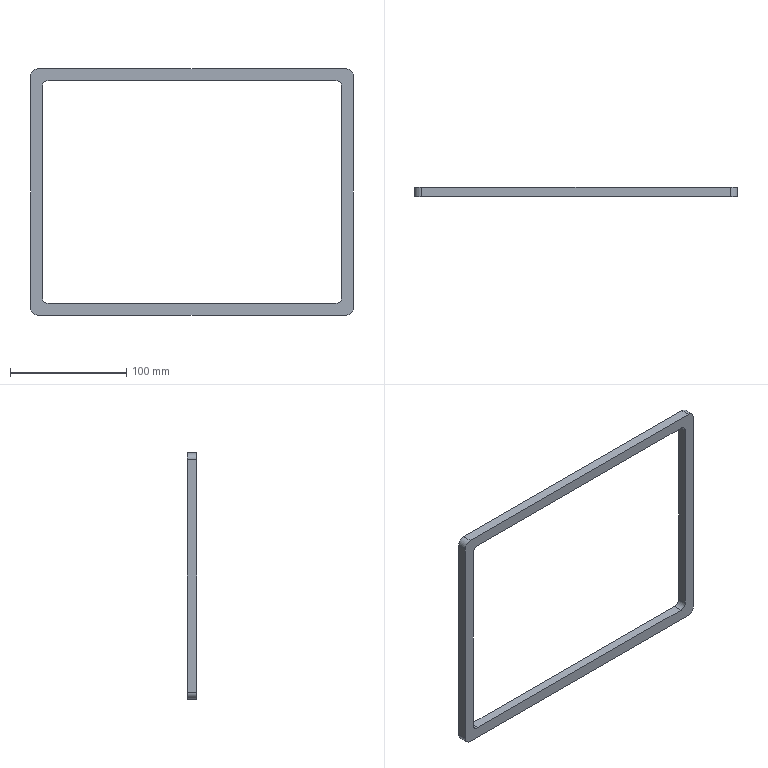Part | NX | 1 solid | 18 faces | box 278 x 8 x 212 mm | volume 75124 mm3 | plane 10 | cylinder 8 | commonest cylinder face diameters 10 x4 12 x4
STEP:
#1=CARTESIAN_POINT('',(-139.,4.,-100.));
#2=VERTEX_POINT('',#1);
#3=CARTESIAN_POINT('',(-133.,4.,-106.));
#4=VERTEX_POINT('',#3);
#5=CARTESIAN_POINT('',(-133.,4.,-100.));
#6=DIRECTION('',(0.,-1.,0.));
#7=DIRECTION('',(0.,0.,-1.));
#8=AXIS2_PLACEMENT_3D('',#5,#6,#7);
#9=CIRCLE('',#8,6.);
#10=EDGE_CURVE('',#2,#4,#9,.T.);
#11=ORIENTED_EDGE('',*,*,#10,.F.);
#12=CARTESIAN_POINT('',(-139.,4.,100.));
#13=VERTEX_POINT('',#12);
#14=CARTESIAN_POINT('',(-139.,4.,100.));
#15=DIRECTION('',(0.,0.,-1.));
#16=VECTOR('',#15,1000.);
#17=LINE('',#14,#16);
#18=EDGE_CURVE('',#13,#2,#17,.T.);
#19=ORIENTED_EDGE('',*,*,#18,.F.);
#20=CARTESIAN_POINT('',(-133.,4.,106.));
#21=VERTEX_POINT('',#20);
#22=CARTESIAN_POINT('',(-133.,4.,100.));
#23=DIRECTION('',(0.,-1.,0.));
#24=DIRECTION('',(0.,0.,-1.));
#25=AXIS2_PLACEMENT_3D('',#22,#23,#24);
#26=CIRCLE('',#25,6.);
#27=EDGE_CURVE('',#21,#13,#26,.T.);
#28=ORIENTED_EDGE('',*,*,#27,.F.);
#29=CARTESIAN_POINT('',(133.,4.,106.));
#30=VERTEX_POINT('',#29);
#31=CARTESIAN_POINT('',(133.,4.,106.));
#32=DIRECTION('',(-1.,0.,0.));
#33=VECTOR('',#32,1000.);
#34=LINE('',#31,#33);
#35=EDGE_CURVE('',#30,#21,#34,.T.);
#36=ORIENTED_EDGE('',*,*,#35,.F.);
#37=CARTESIAN_POINT('',(139.,4.,100.));
#38=VERTEX_POINT('',#37);
#39=CARTESIAN_POINT('',(133.,4.,100.));
#40=DIRECTION('',(0.,-1.,0.));
#41=DIRECTION('',(0.,0.,-1.));
#42=AXIS2_PLACEMENT_3D('',#39,#40,#41);
#43=CIRCLE('',#42,6.);
#44=EDGE_CURVE('',#38,#30,#43,.T.);
#45=ORIENTED_EDGE('',*,*,#44,.F.);
#46=CARTESIAN_POINT('',(139.,4.,-100.));
#47=VERTEX_POINT('',#46);
#48=CARTESIAN_POINT('',(139.,4.,-100.));
#49=DIRECTION('',(0.,0.,1.));
#50=VECTOR('',#49,1000.);
#51=LINE('',#48,#50);
#52=EDGE_CURVE('',#47,#38,#51,.T.);
#53=ORIENTED_EDGE('',*,*,#52,.F.);
#54=CARTESIAN_POINT('',(133.,4.,-106.));
#55=VERTEX_POINT('',#54);
#56=CARTESIAN_POINT('',(133.,4.,-100.));
#57=DIRECTION('',(0.,-1.,0.));
#58=DIRECTION('',(0.,0.,-1.));
#59=AXIS2_PLACEMENT_3D('',#56,#57,#58);
#60=CIRCLE('',#59,6.);
#61=EDGE_CURVE('',#55,#47,#60,.T.);
#62=ORIENTED_EDGE('',*,*,#61,.F.);
#63=CARTESIAN_POINT('',(-133.,4.,-106.));
#64=DIRECTION('',(1.,0.,0.));
#65=VECTOR('',#64,1000.);
#66=LINE('',#63,#65);
#67=EDGE_CURVE('',#4,#55,#66,.T.);
#68=ORIENTED_EDGE('',*,*,#67,.F.);
#69=EDGE_LOOP('',(#11,#19,#28,#36,#45,#53,#62,#68));
#70=FACE_BOUND('',#69,.T.);
#71=CARTESIAN_POINT('',(-129.,4.,-91.));
#72=VERTEX_POINT('',#71);
#73=CARTESIAN_POINT('',(-124.,4.,-96.));
#74=VERTEX_POINT('',#73);
#75=CARTESIAN_POINT('',(-124.,4.,-91.));
#76=DIRECTION('',(0.,-1.,0.));
#77=DIRECTION('',(0.,0.,-1.));
#78=AXIS2_PLACEMENT_3D('',#75,#76,#77);
#79=CIRCLE('',#78,5.);
#80=EDGE_CURVE('',#72,#74,#79,.T.);
#81=ORIENTED_EDGE('',*,*,#80,.T.);
#82=CARTESIAN_POINT('',(124.,4.,-96.));
#83=VERTEX_POINT('',#82);
#84=CARTESIAN_POINT('',(-124.,4.,-96.));
#85=DIRECTION('',(1.,0.,0.));
#86=VECTOR('',#85,1000.);
#87=LINE('',#84,#86);
#88=EDGE_CURVE('',#74,#83,#87,.T.);
#89=ORIENTED_EDGE('',*,*,#88,.T.);
#90=CARTESIAN_POINT('',(129.,4.,-91.));
#91=VERTEX_POINT('',#90);
#92=CARTESIAN_POINT('',(124.,4.,-91.));
#93=DIRECTION('',(0.,-1.,0.));
#94=DIRECTION('',(0.,0.,-1.));
#95=AXIS2_PLACEMENT_3D('',#92,#93,#94);
#96=CIRCLE('',#95,5.);
#97=EDGE_CURVE('',#83,#91,#96,.T.);
#98=ORIENTED_EDGE('',*,*,#97,.T.);
#99=CARTESIAN_POINT('',(129.,4.,91.));
#100=VERTEX_POINT('',#99);
#101=CARTESIAN_POINT('',(129.,4.,-91.));
#102=DIRECTION('',(0.,0.,1.));
#103=VECTOR('',#102,1000.);
#104=LINE('',#101,#103);
#105=EDGE_CURVE('',#91,#100,#104,.T.);
#106=ORIENTED_EDGE('',*,*,#105,.T.);
#107=CARTESIAN_POINT('',(124.,4.,96.));
#108=VERTEX_POINT('',#107);
#109=CARTESIAN_POINT('',(124.,4.,91.));
#110=DIRECTION('',(0.,-1.,0.));
#111=DIRECTION('',(0.,0.,-1.));
#112=AXIS2_PLACEMENT_3D('',#109,#110,#111);
#113=CIRCLE('',#112,5.);
#114=EDGE_CURVE('',#100,#108,#113,.T.);
#115=ORIENTED_EDGE('',*,*,#114,.T.);
#116=CARTESIAN_POINT('',(-124.,4.,96.));
#117=VERTEX_POINT('',#116);
#118=CARTESIAN_POINT('',(124.,4.,96.));
#119=DIRECTION('',(-1.,0.,0.));
#120=VECTOR('',#119,1000.);
#121=LINE('',#118,#120);
#122=EDGE_CURVE('',#108,#117,#121,.T.);
#123=ORIENTED_EDGE('',*,*,#122,.T.);
#124=CARTESIAN_POINT('',(-129.,4.,91.));
#125=VERTEX_POINT('',#124);
#126=CARTESIAN_POINT('',(-124.,4.,91.));
#127=DIRECTION('',(0.,-1.,0.));
#128=DIRECTION('',(0.,0.,-1.));
#129=AXIS2_PLACEMENT_3D('',#126,#127,#128);
#130=CIRCLE('',#129,5.);
#131=EDGE_CURVE('',#117,#125,#130,.T.);
#132=ORIENTED_EDGE('',*,*,#131,.T.);
#133=CARTESIAN_POINT('',(-129.,4.,91.));
#134=DIRECTION('',(0.,0.,-1.));
#135=VECTOR('',#134,1000.);
#136=LINE('',#133,#135);
#137=EDGE_CURVE('',#125,#72,#136,.T.);
#138=ORIENTED_EDGE('',*,*,#137,.T.);
#139=EDGE_LOOP('',(#81,#89,#98,#106,#115,#123,#132,#138));
#140=FACE_BOUND('',#139,.T.);
#141=CARTESIAN_POINT('',(-133.,4.,-100.));
#142=DIRECTION('',(0.,-1.,0.));
#143=DIRECTION('',(0.,0.,-1.));
#144=AXIS2_PLACEMENT_3D('',#141,#142,#143);
#145=PLANE('',#144);
#146=ADVANCED_FACE('',(#70,#140),#145,.F.);
#147=CARTESIAN_POINT('',(-133.,-4.,-106.));
#148=VERTEX_POINT('',#147);
#149=CARTESIAN_POINT('',(-133.,-353.611,-106.));
#150=DIRECTION('',(0.,1.,0.));
#151=VECTOR('',#150,1000.);
#152=LINE('',#149,#151);
#153=EDGE_CURVE('',#148,#4,#152,.T.);
#154=ORIENTED_EDGE('',*,*,#153,.F.);
#155=CARTESIAN_POINT('',(-139.,-4.,-100.));
#156=VERTEX_POINT('',#155);
#157=CARTESIAN_POINT('',(-133.,-4.,-100.));
#158=DIRECTION('',(0.,1.,0.));
#159=DIRECTION('',(0.,0.,1.));
#160=AXIS2_PLACEMENT_3D('',#157,#158,#159);
#161=CIRCLE('',#160,6.);
#162=EDGE_CURVE('',#148,#156,#161,.T.);
#163=ORIENTED_EDGE('',*,*,#162,.T.);
#164=CARTESIAN_POINT('',(-139.,-353.611,-100.));
#165=DIRECTION('',(0.,1.,0.));
#166=VECTOR('',#165,1000.);
#167=LINE('',#164,#166);
#168=EDGE_CURVE('',#156,#2,#167,.T.);
#169=ORIENTED_EDGE('',*,*,#168,.T.);
#170=ORIENTED_EDGE('',*,*,#10,.T.);
#171=EDGE_LOOP('',(#154,#163,#169,#170));
#172=FACE_BOUND('',#171,.T.);
#173=CARTESIAN_POINT('',(-133.,-353.611,-100.));
#174=DIRECTION('',(0.,1.,0.));
#175=DIRECTION('',(0.,0.,1.));
#176=AXIS2_PLACEMENT_3D('',#173,#174,#175);
#177=CYLINDRICAL_SURFACE('',#176,6.);
#178=ADVANCED_FACE('',(#172),#177,.T.);
#179=CARTESIAN_POINT('',(133.,-4.,-106.));
#180=VERTEX_POINT('',#179);
#181=CARTESIAN_POINT('',(133.,-353.611,-106.));
#182=DIRECTION('',(0.,1.,0.));
#183=VECTOR('',#182,1000.);
#184=LINE('',#181,#183);
#185=EDGE_CURVE('',#180,#55,#184,.T.);
#186=ORIENTED_EDGE('',*,*,#185,.F.);
#187=CARTESIAN_POINT('',(-133.,-4.,-106.));
#188=DIRECTION('',(-1.,0.,0.));
#189=VECTOR('',#188,1000.);
#190=LINE('',#187,#189);
#191=EDGE_CURVE('',#180,#148,#190,.T.);
#192=ORIENTED_EDGE('',*,*,#191,.T.);
#193=ORIENTED_EDGE('',*,*,#153,.T.);
#194=ORIENTED_EDGE('',*,*,#67,.T.);
#195=EDGE_LOOP('',(#186,#192,#193,#194));
#196=FACE_BOUND('',#195,.T.);
#197=CARTESIAN_POINT('',(-133.,-353.611,-106.));
#198=DIRECTION('',(0.,0.,1.));
#199=DIRECTION('',(1.,0.,0.));
#200=AXIS2_PLACEMENT_3D('',#197,#198,#199);
#201=PLANE('',#200);
#202=ADVANCED_FACE('',(#196),#201,.F.);
#203=CARTESIAN_POINT('',(139.,-4.,-100.));
#204=VERTEX_POINT('',#203);
#205=CARTESIAN_POINT('',(139.,-353.611,-100.));
#206=DIRECTION('',(0.,1.,0.));
#207=VECTOR('',#206,1000.);
#208=LINE('',#205,#207);
#209=EDGE_CURVE('',#204,#47,#208,.T.);
#210=ORIENTED_EDGE('',*,*,#209,.F.);
#211=CARTESIAN_POINT('',(133.,-4.,-100.));
#212=DIRECTION('',(0.,1.,0.));
#213=DIRECTION('',(0.,0.,1.));
#214=AXIS2_PLACEMENT_3D('',#211,#212,#213);
#215=CIRCLE('',#214,6.);
#216=EDGE_CURVE('',#204,#180,#215,.T.);
#217=ORIENTED_EDGE('',*,*,#216,.T.);
#218=ORIENTED_EDGE('',*,*,#185,.T.);
#219=ORIENTED_EDGE('',*,*,#61,.T.);
#220=EDGE_LOOP('',(#210,#217,#218,#219));
#221=FACE_BOUND('',#220,.T.);
#222=CARTESIAN_POINT('',(133.,-353.611,-100.));
#223=DIRECTION('',(0.,1.,0.));
#224=DIRECTION('',(0.,0.,1.));
#225=AXIS2_PLACEMENT_3D('',#222,#223,#224);
#226=CYLINDRICAL_SURFACE('',#225,6.);
#227=ADVANCED_FACE('',(#221),#226,.T.);
#228=CARTESIAN_POINT('',(139.,-4.,100.));
#229=VERTEX_POINT('',#228);
#230=CARTESIAN_POINT('',(139.,-353.611,100.));
#231=DIRECTION('',(0.,1.,0.));
#232=VECTOR('',#231,1000.);
#233=LINE('',#230,#232);
#234=EDGE_CURVE('',#229,#38,#233,.T.);
#235=ORIENTED_EDGE('',*,*,#234,.F.);
#236=CARTESIAN_POINT('',(139.,-4.,-100.));
#237=DIRECTION('',(0.,0.,-1.));
#238=VECTOR('',#237,1000.);
#239=LINE('',#236,#238);
#240=EDGE_CURVE('',#229,#204,#239,.T.);
#241=ORIENTED_EDGE('',*,*,#240,.T.);
#242=ORIENTED_EDGE('',*,*,#209,.T.);
#243=ORIENTED_EDGE('',*,*,#52,.T.);
#244=EDGE_LOOP('',(#235,#241,#242,#243));
#245=FACE_BOUND('',#244,.T.);
#246=CARTESIAN_POINT('',(139.,-353.611,-100.));
#247=DIRECTION('',(-1.,0.,0.));
#248=DIRECTION('',(0.,0.,1.));
#249=AXIS2_PLACEMENT_3D('',#246,#247,#248);
#250=PLANE('',#249);
#251=ADVANCED_FACE('',(#245),#250,.F.);
#252=CARTESIAN_POINT('',(133.,-4.,106.));
#253=VERTEX_POINT('',#252);
#254=CARTESIAN_POINT('',(133.,-353.611,106.));
#255=DIRECTION('',(0.,1.,0.));
#256=VECTOR('',#255,1000.);
#257=LINE('',#254,#256);
#258=EDGE_CURVE('',#253,#30,#257,.T.);
#259=ORIENTED_EDGE('',*,*,#258,.F.);
#260=CARTESIAN_POINT('',(133.,-4.,100.));
#261=DIRECTION('',(0.,1.,0.));
#262=DIRECTION('',(0.,0.,1.));
#263=AXIS2_PLACEMENT_3D('',#260,#261,#262);
#264=CIRCLE('',#263,6.);
#265=EDGE_CURVE('',#253,#229,#264,.T.);
#266=ORIENTED_EDGE('',*,*,#265,.T.);
#267=ORIENTED_EDGE('',*,*,#234,.T.);
#268=ORIENTED_EDGE('',*,*,#44,.T.);
#269=EDGE_LOOP('',(#259,#266,#267,#268));
#270=FACE_BOUND('',#269,.T.);
#271=CARTESIAN_POINT('',(133.,-353.611,100.));
#272=DIRECTION('',(0.,1.,0.));
#273=DIRECTION('',(0.,0.,1.));
#274=AXIS2_PLACEMENT_3D('',#271,#272,#273);
#275=CYLINDRICAL_SURFACE('',#274,6.);
#276=ADVANCED_FACE('',(#270),#275,.T.);
#277=CARTESIAN_POINT('',(-133.,-4.,106.));
#278=VERTEX_POINT('',#277);
#279=CARTESIAN_POINT('',(-133.,-353.611,106.));
#280=DIRECTION('',(0.,1.,0.));
#281=VECTOR('',#280,1000.);
#282=LINE('',#279,#281);
#283=EDGE_CURVE('',#278,#21,#282,.T.);
#284=ORIENTED_EDGE('',*,*,#283,.F.);
#285=CARTESIAN_POINT('',(133.,-4.,106.));
#286=DIRECTION('',(1.,0.,0.));
#287=VECTOR('',#286,1000.);
#288=LINE('',#285,#287);
#289=EDGE_CURVE('',#278,#253,#288,.T.);
#290=ORIENTED_EDGE('',*,*,#289,.T.);
#291=ORIENTED_EDGE('',*,*,#258,.T.);
#292=ORIENTED_EDGE('',*,*,#35,.T.);
#293=EDGE_LOOP('',(#284,#290,#291,#292));
#294=FACE_BOUND('',#293,.T.);
#295=CARTESIAN_POINT('',(133.,-353.611,106.));
#296=DIRECTION('',(0.,0.,-1.));
#297=DIRECTION('',(-1.,0.,0.));
#298=AXIS2_PLACEMENT_3D('',#295,#296,#297);
#299=PLANE('',#298);
#300=ADVANCED_FACE('',(#294),#299,.F.);
#301=CARTESIAN_POINT('',(-139.,-4.,100.));
#302=VERTEX_POINT('',#301);
#303=CARTESIAN_POINT('',(-139.,-353.611,100.));
#304=DIRECTION('',(0.,1.,0.));
#305=VECTOR('',#304,1000.);
#306=LINE('',#303,#305);
#307=EDGE_CURVE('',#302,#13,#306,.T.);
#308=ORIENTED_EDGE('',*,*,#307,.F.);
#309=CARTESIAN_POINT('',(-133.,-4.,100.));
#310=DIRECTION('',(0.,1.,0.));
#311=DIRECTION('',(0.,0.,1.));
#312=AXIS2_PLACEMENT_3D('',#309,#310,#311);
#313=CIRCLE('',#312,6.);
#314=EDGE_CURVE('',#302,#278,#313,.T.);
#315=ORIENTED_EDGE('',*,*,#314,.T.);
#316=ORIENTED_EDGE('',*,*,#283,.T.);
#317=ORIENTED_EDGE('',*,*,#27,.T.);
#318=EDGE_LOOP('',(#308,#315,#316,#317));
#319=FACE_BOUND('',#318,.T.);
#320=CARTESIAN_POINT('',(-133.,-353.611,100.));
#321=DIRECTION('',(0.,1.,0.));
#322=DIRECTION('',(0.,0.,1.));
#323=AXIS2_PLACEMENT_3D('',#320,#321,#322);
#324=CYLINDRICAL_SURFACE('',#323,6.);
#325=ADVANCED_FACE('',(#319),#324,.T.);
#326=ORIENTED_EDGE('',*,*,#168,.F.);
#327=CARTESIAN_POINT('',(-139.,-4.,100.));
#328=DIRECTION('',(0.,0.,1.));
#329=VECTOR('',#328,1000.);
#330=LINE('',#327,#329);
#331=EDGE_CURVE('',#156,#302,#330,.T.);
#332=ORIENTED_EDGE('',*,*,#331,.T.);
#333=ORIENTED_EDGE('',*,*,#307,.T.);
#334=ORIENTED_EDGE('',*,*,#18,.T.);
#335=EDGE_LOOP('',(#326,#332,#333,#334));
#336=FACE_BOUND('',#335,.T.);
#337=CARTESIAN_POINT('',(-139.,-353.611,100.));
#338=DIRECTION('',(1.,0.,0.));
#339=DIRECTION('',(0.,0.,-1.));
#340=AXIS2_PLACEMENT_3D('',#337,#338,#339);
#341=PLANE('',#340);
#342=ADVANCED_FACE('',(#336),#341,.F.);
#343=CARTESIAN_POINT('',(-124.,-4.,-96.));
#344=VERTEX_POINT('',#343);
#345=CARTESIAN_POINT('',(-129.,-4.,-91.));
#346=VERTEX_POINT('',#345);
#347=CARTESIAN_POINT('',(-124.,-4.,-91.));
#348=DIRECTION('',(0.,1.,0.));
#349=DIRECTION('',(0.,0.,1.));
#350=AXIS2_PLACEMENT_3D('',#347,#348,#349);
#351=CIRCLE('',#350,5.);
#352=EDGE_CURVE('',#344,#346,#351,.T.);
#353=ORIENTED_EDGE('',*,*,#352,.F.);
#354=CARTESIAN_POINT('',(-124.,-353.611,-96.));
#355=DIRECTION('',(0.,1.,0.));
#356=VECTOR('',#355,1000.);
#357=LINE('',#354,#356);
#358=EDGE_CURVE('',#344,#74,#357,.T.);
#359=ORIENTED_EDGE('',*,*,#358,.T.);
#360=ORIENTED_EDGE('',*,*,#80,.F.);
#361=CARTESIAN_POINT('',(-129.,-353.611,-91.));
#362=DIRECTION('',(0.,1.,0.));
#363=VECTOR('',#362,1000.);
#364=LINE('',#361,#363);
#365=EDGE_CURVE('',#346,#72,#364,.T.);
#366=ORIENTED_EDGE('',*,*,#365,.F.);
#367=EDGE_LOOP('',(#353,#359,#360,#366));
#368=FACE_BOUND('',#367,.T.);
#369=CARTESIAN_POINT('',(-124.,-353.611,-91.));
#370=DIRECTION('',(0.,1.,0.));
#371=DIRECTION('',(0.,0.,1.));
#372=AXIS2_PLACEMENT_3D('',#369,#370,#371);
#373=CYLINDRICAL_SURFACE('',#372,5.);
#374=ADVANCED_FACE('',(#368),#373,.F.);
#375=CARTESIAN_POINT('',(124.,-4.,-96.));
#376=VERTEX_POINT('',#375);
#377=CARTESIAN_POINT('',(-124.,-4.,-96.));
#378=DIRECTION('',(-1.,0.,0.));
#379=VECTOR('',#378,1000.);
#380=LINE('',#377,#379);
#381=EDGE_CURVE('',#376,#344,#380,.T.);
#382=ORIENTED_EDGE('',*,*,#381,.F.);
#383=CARTESIAN_POINT('',(124.,-353.611,-96.));
#384=DIRECTION('',(0.,1.,0.));
#385=VECTOR('',#384,1000.);
#386=LINE('',#383,#385);
#387=EDGE_CURVE('',#376,#83,#386,.T.);
#388=ORIENTED_EDGE('',*,*,#387,.T.);
#389=ORIENTED_EDGE('',*,*,#88,.F.);
#390=ORIENTED_EDGE('',*,*,#358,.F.);
#391=EDGE_LOOP('',(#382,#388,#389,#390));
#392=FACE_BOUND('',#391,.T.);
#393=CARTESIAN_POINT('',(-124.,-353.611,-96.));
#394=DIRECTION('',(0.,0.,1.));
#395=DIRECTION('',(1.,0.,0.));
#396=AXIS2_PLACEMENT_3D('',#393,#394,#395);
#397=PLANE('',#396);
#398=ADVANCED_FACE('',(#392),#397,.T.);
#399=CARTESIAN_POINT('',(129.,-4.,-91.));
#400=VERTEX_POINT('',#399);
#401=CARTESIAN_POINT('',(124.,-4.,-91.));
#402=DIRECTION('',(0.,1.,0.));
#403=DIRECTION('',(0.,0.,1.));
#404=AXIS2_PLACEMENT_3D('',#401,#402,#403);
#405=CIRCLE('',#404,5.);
#406=EDGE_CURVE('',#400,#376,#405,.T.);
#407=ORIENTED_EDGE('',*,*,#406,.F.);
#408=CARTESIAN_POINT('',(129.,-353.611,-91.));
#409=DIRECTION('',(0.,1.,0.));
#410=VECTOR('',#409,1000.);
#411=LINE('',#408,#410);
#412=EDGE_CURVE('',#400,#91,#411,.T.);
#413=ORIENTED_EDGE('',*,*,#412,.T.);
#414=ORIENTED_EDGE('',*,*,#97,.F.);
#415=ORIENTED_EDGE('',*,*,#387,.F.);
#416=EDGE_LOOP('',(#407,#413,#414,#415));
#417=FACE_BOUND('',#416,.T.);
#418=CARTESIAN_POINT('',(124.,-353.611,-91.));
#419=DIRECTION('',(0.,1.,0.));
#420=DIRECTION('',(0.,0.,1.));
#421=AXIS2_PLACEMENT_3D('',#418,#419,#420);
#422=CYLINDRICAL_SURFACE('',#421,5.);
#423=ADVANCED_FACE('',(#417),#422,.F.);
#424=CARTESIAN_POINT('',(129.,-4.,91.));
#425=VERTEX_POINT('',#424);
#426=CARTESIAN_POINT('',(129.,-4.,-91.));
#427=DIRECTION('',(0.,0.,-1.));
#428=VECTOR('',#427,1000.);
#429=LINE('',#426,#428);
#430=EDGE_CURVE('',#425,#400,#429,.T.);
#431=ORIENTED_EDGE('',*,*,#430,.F.);
#432=CARTESIAN_POINT('',(129.,-353.611,91.));
#433=DIRECTION('',(0.,1.,0.));
#434=VECTOR('',#433,1000.);
#435=LINE('',#432,#434);
#436=EDGE_CURVE('',#425,#100,#435,.T.);
#437=ORIENTED_EDGE('',*,*,#436,.T.);
#438=ORIENTED_EDGE('',*,*,#105,.F.);
#439=ORIENTED_EDGE('',*,*,#412,.F.);
#440=EDGE_LOOP('',(#431,#437,#438,#439));
#441=FACE_BOUND('',#440,.T.);
#442=CARTESIAN_POINT('',(129.,-353.611,-91.));
#443=DIRECTION('',(-1.,0.,0.));
#444=DIRECTION('',(0.,0.,1.));
#445=AXIS2_PLACEMENT_3D('',#442,#443,#444);
#446=PLANE('',#445);
#447=ADVANCED_FACE('',(#441),#446,.T.);
#448=CARTESIAN_POINT('',(124.,-4.,96.));
#449=VERTEX_POINT('',#448);
#450=CARTESIAN_POINT('',(124.,-4.,91.));
#451=DIRECTION('',(0.,1.,0.));
#452=DIRECTION('',(0.,0.,1.));
#453=AXIS2_PLACEMENT_3D('',#450,#451,#452);
#454=CIRCLE('',#453,5.);
#455=EDGE_CURVE('',#449,#425,#454,.T.);
#456=ORIENTED_EDGE('',*,*,#455,.F.);
#457=CARTESIAN_POINT('',(124.,-353.611,96.));
#458=DIRECTION('',(0.,1.,0.));
#459=VECTOR('',#458,1000.);
#460=LINE('',#457,#459);
#461=EDGE_CURVE('',#449,#108,#460,.T.);
#462=ORIENTED_EDGE('',*,*,#461,.T.);
#463=ORIENTED_EDGE('',*,*,#114,.F.);
#464=ORIENTED_EDGE('',*,*,#436,.F.);
#465=EDGE_LOOP('',(#456,#462,#463,#464));
#466=FACE_BOUND('',#465,.T.);
#467=CARTESIAN_POINT('',(124.,-353.611,91.));
#468=DIRECTION('',(0.,1.,0.));
#469=DIRECTION('',(0.,0.,1.));
#470=AXIS2_PLACEMENT_3D('',#467,#468,#469);
#471=CYLINDRICAL_SURFACE('',#470,5.);
#472=ADVANCED_FACE('',(#466),#471,.F.);
#473=CARTESIAN_POINT('',(-124.,-4.,96.));
#474=VERTEX_POINT('',#473);
#475=CARTESIAN_POINT('',(124.,-4.,96.));
#476=DIRECTION('',(1.,0.,0.));
#477=VECTOR('',#476,1000.);
#478=LINE('',#475,#477);
#479=EDGE_CURVE('',#474,#449,#478,.T.);
#480=ORIENTED_EDGE('',*,*,#479,.F.);
#481=CARTESIAN_POINT('',(-124.,-353.611,96.));
#482=DIRECTION('',(0.,1.,0.));
#483=VECTOR('',#482,1000.);
#484=LINE('',#481,#483);
#485=EDGE_CURVE('',#474,#117,#484,.T.);
#486=ORIENTED_EDGE('',*,*,#485,.T.);
#487=ORIENTED_EDGE('',*,*,#122,.F.);
#488=ORIENTED_EDGE('',*,*,#461,.F.);
#489=EDGE_LOOP('',(#480,#486,#487,#488));
#490=FACE_BOUND('',#489,.T.);
#491=CARTESIAN_POINT('',(124.,-353.611,96.));
#492=DIRECTION('',(0.,0.,-1.));
#493=DIRECTION('',(-1.,0.,0.));
#494=AXIS2_PLACEMENT_3D('',#491,#492,#493);
#495=PLANE('',#494);
#496=ADVANCED_FACE('',(#490),#495,.T.);
#497=CARTESIAN_POINT('',(-129.,-4.,91.));
#498=VERTEX_POINT('',#497);
#499=CARTESIAN_POINT('',(-124.,-4.,91.));
#500=DIRECTION('',(0.,1.,0.));
#501=DIRECTION('',(0.,0.,1.));
#502=AXIS2_PLACEMENT_3D('',#499,#500,#501);
#503=CIRCLE('',#502,5.);
#504=EDGE_CURVE('',#498,#474,#503,.T.);
#505=ORIENTED_EDGE('',*,*,#504,.F.);
#506=CARTESIAN_POINT('',(-129.,-353.611,91.));
#507=DIRECTION('',(0.,1.,0.));
#508=VECTOR('',#507,1000.);
#509=LINE('',#506,#508);
#510=EDGE_CURVE('',#498,#125,#509,.T.);
#511=ORIENTED_EDGE('',*,*,#510,.T.);
#512=ORIENTED_EDGE('',*,*,#131,.F.);
#513=ORIENTED_EDGE('',*,*,#485,.F.);
#514=EDGE_LOOP('',(#505,#511,#512,#513));
#515=FACE_BOUND('',#514,.T.);
#516=CARTESIAN_POINT('',(-124.,-353.611,91.));
#517=DIRECTION('',(0.,1.,0.));
#518=DIRECTION('',(0.,0.,1.));
#519=AXIS2_PLACEMENT_3D('',#516,#517,#518);
#520=CYLINDRICAL_SURFACE('',#519,5.);
#521=ADVANCED_FACE('',(#515),#520,.F.);
#522=CARTESIAN_POINT('',(-129.,-4.,91.));
#523=DIRECTION('',(0.,0.,1.));
#524=VECTOR('',#523,1000.);
#525=LINE('',#522,#524);
#526=EDGE_CURVE('',#346,#498,#525,.T.);
#527=ORIENTED_EDGE('',*,*,#526,.F.);
#528=ORIENTED_EDGE('',*,*,#365,.T.);
#529=ORIENTED_EDGE('',*,*,#137,.F.);
#530=ORIENTED_EDGE('',*,*,#510,.F.);
#531=EDGE_LOOP('',(#527,#528,#529,#530));
#532=FACE_BOUND('',#531,.T.);
#533=CARTESIAN_POINT('',(-129.,-353.611,91.));
#534=DIRECTION('',(1.,0.,0.));
#535=DIRECTION('',(0.,0.,-1.));
#536=AXIS2_PLACEMENT_3D('',#533,#534,#535);
#537=PLANE('',#536);
#538=ADVANCED_FACE('',(#532),#537,.T.);
#539=ORIENTED_EDGE('',*,*,#352,.T.);
#540=ORIENTED_EDGE('',*,*,#526,.T.);
#541=ORIENTED_EDGE('',*,*,#504,.T.);
#542=ORIENTED_EDGE('',*,*,#479,.T.);
#543=ORIENTED_EDGE('',*,*,#455,.T.);
#544=ORIENTED_EDGE('',*,*,#430,.T.);
#545=ORIENTED_EDGE('',*,*,#406,.T.);
#546=ORIENTED_EDGE('',*,*,#381,.T.);
#547=EDGE_LOOP('',(#539,#540,#541,#542,#543,#544,#545,#546));
#548=FACE_BOUND('',#547,.T.);
#549=ORIENTED_EDGE('',*,*,#191,.F.);
#550=ORIENTED_EDGE('',*,*,#216,.F.);
#551=ORIENTED_EDGE('',*,*,#240,.F.);
#552=ORIENTED_EDGE('',*,*,#265,.F.);
#553=ORIENTED_EDGE('',*,*,#289,.F.);
#554=ORIENTED_EDGE('',*,*,#314,.F.);
#555=ORIENTED_EDGE('',*,*,#331,.F.);
#556=ORIENTED_EDGE('',*,*,#162,.F.);
#557=EDGE_LOOP('',(#549,#550,#551,#552,#553,#554,#555,#556));
#558=FACE_BOUND('',#557,.T.);
#559=CARTESIAN_POINT('',(0.,-4.,0.));
#560=DIRECTION('',(0.,1.,0.));
#561=DIRECTION('',(0.,0.,1.));
#562=AXIS2_PLACEMENT_3D('',#559,#560,#561);
#563=PLANE('',#562);
#564=ADVANCED_FACE('',(#548,#558),#563,.F.);
#565=CLOSED_SHELL('',(#146,#178,#202,#227,#251,#276,#300,#325,#342,#374,#398,#423,#447,#472,#496,#521,#538,#564));
#566=MANIFOLD_SOLID_BREP('',#565);
#567=(LENGTH_UNIT()NAMED_UNIT(*)SI_UNIT(.MILLI.,.METRE.));
#568=UNCERTAINTY_MEASURE_WITH_UNIT(LENGTH_MEASURE(0.00001),#567,'','');
#569=(NAMED_UNIT(*)PLANE_ANGLE_UNIT()SI_UNIT($,.RADIAN.));
#570=(NAMED_UNIT(*)SI_UNIT($,.STERADIAN.)SOLID_ANGLE_UNIT());
#571=(GEOMETRIC_REPRESENTATION_CONTEXT(3)GLOBAL_UNCERTAINTY_ASSIGNED_CONTEXT((#568))GLOBAL_UNIT_ASSIGNED_CONTEXT((#567,#569,#570))REPRESENTATION_CONTEXT('',''));
#572=ADVANCED_BREP_SHAPE_REPRESENTATION('',(#566),#571);